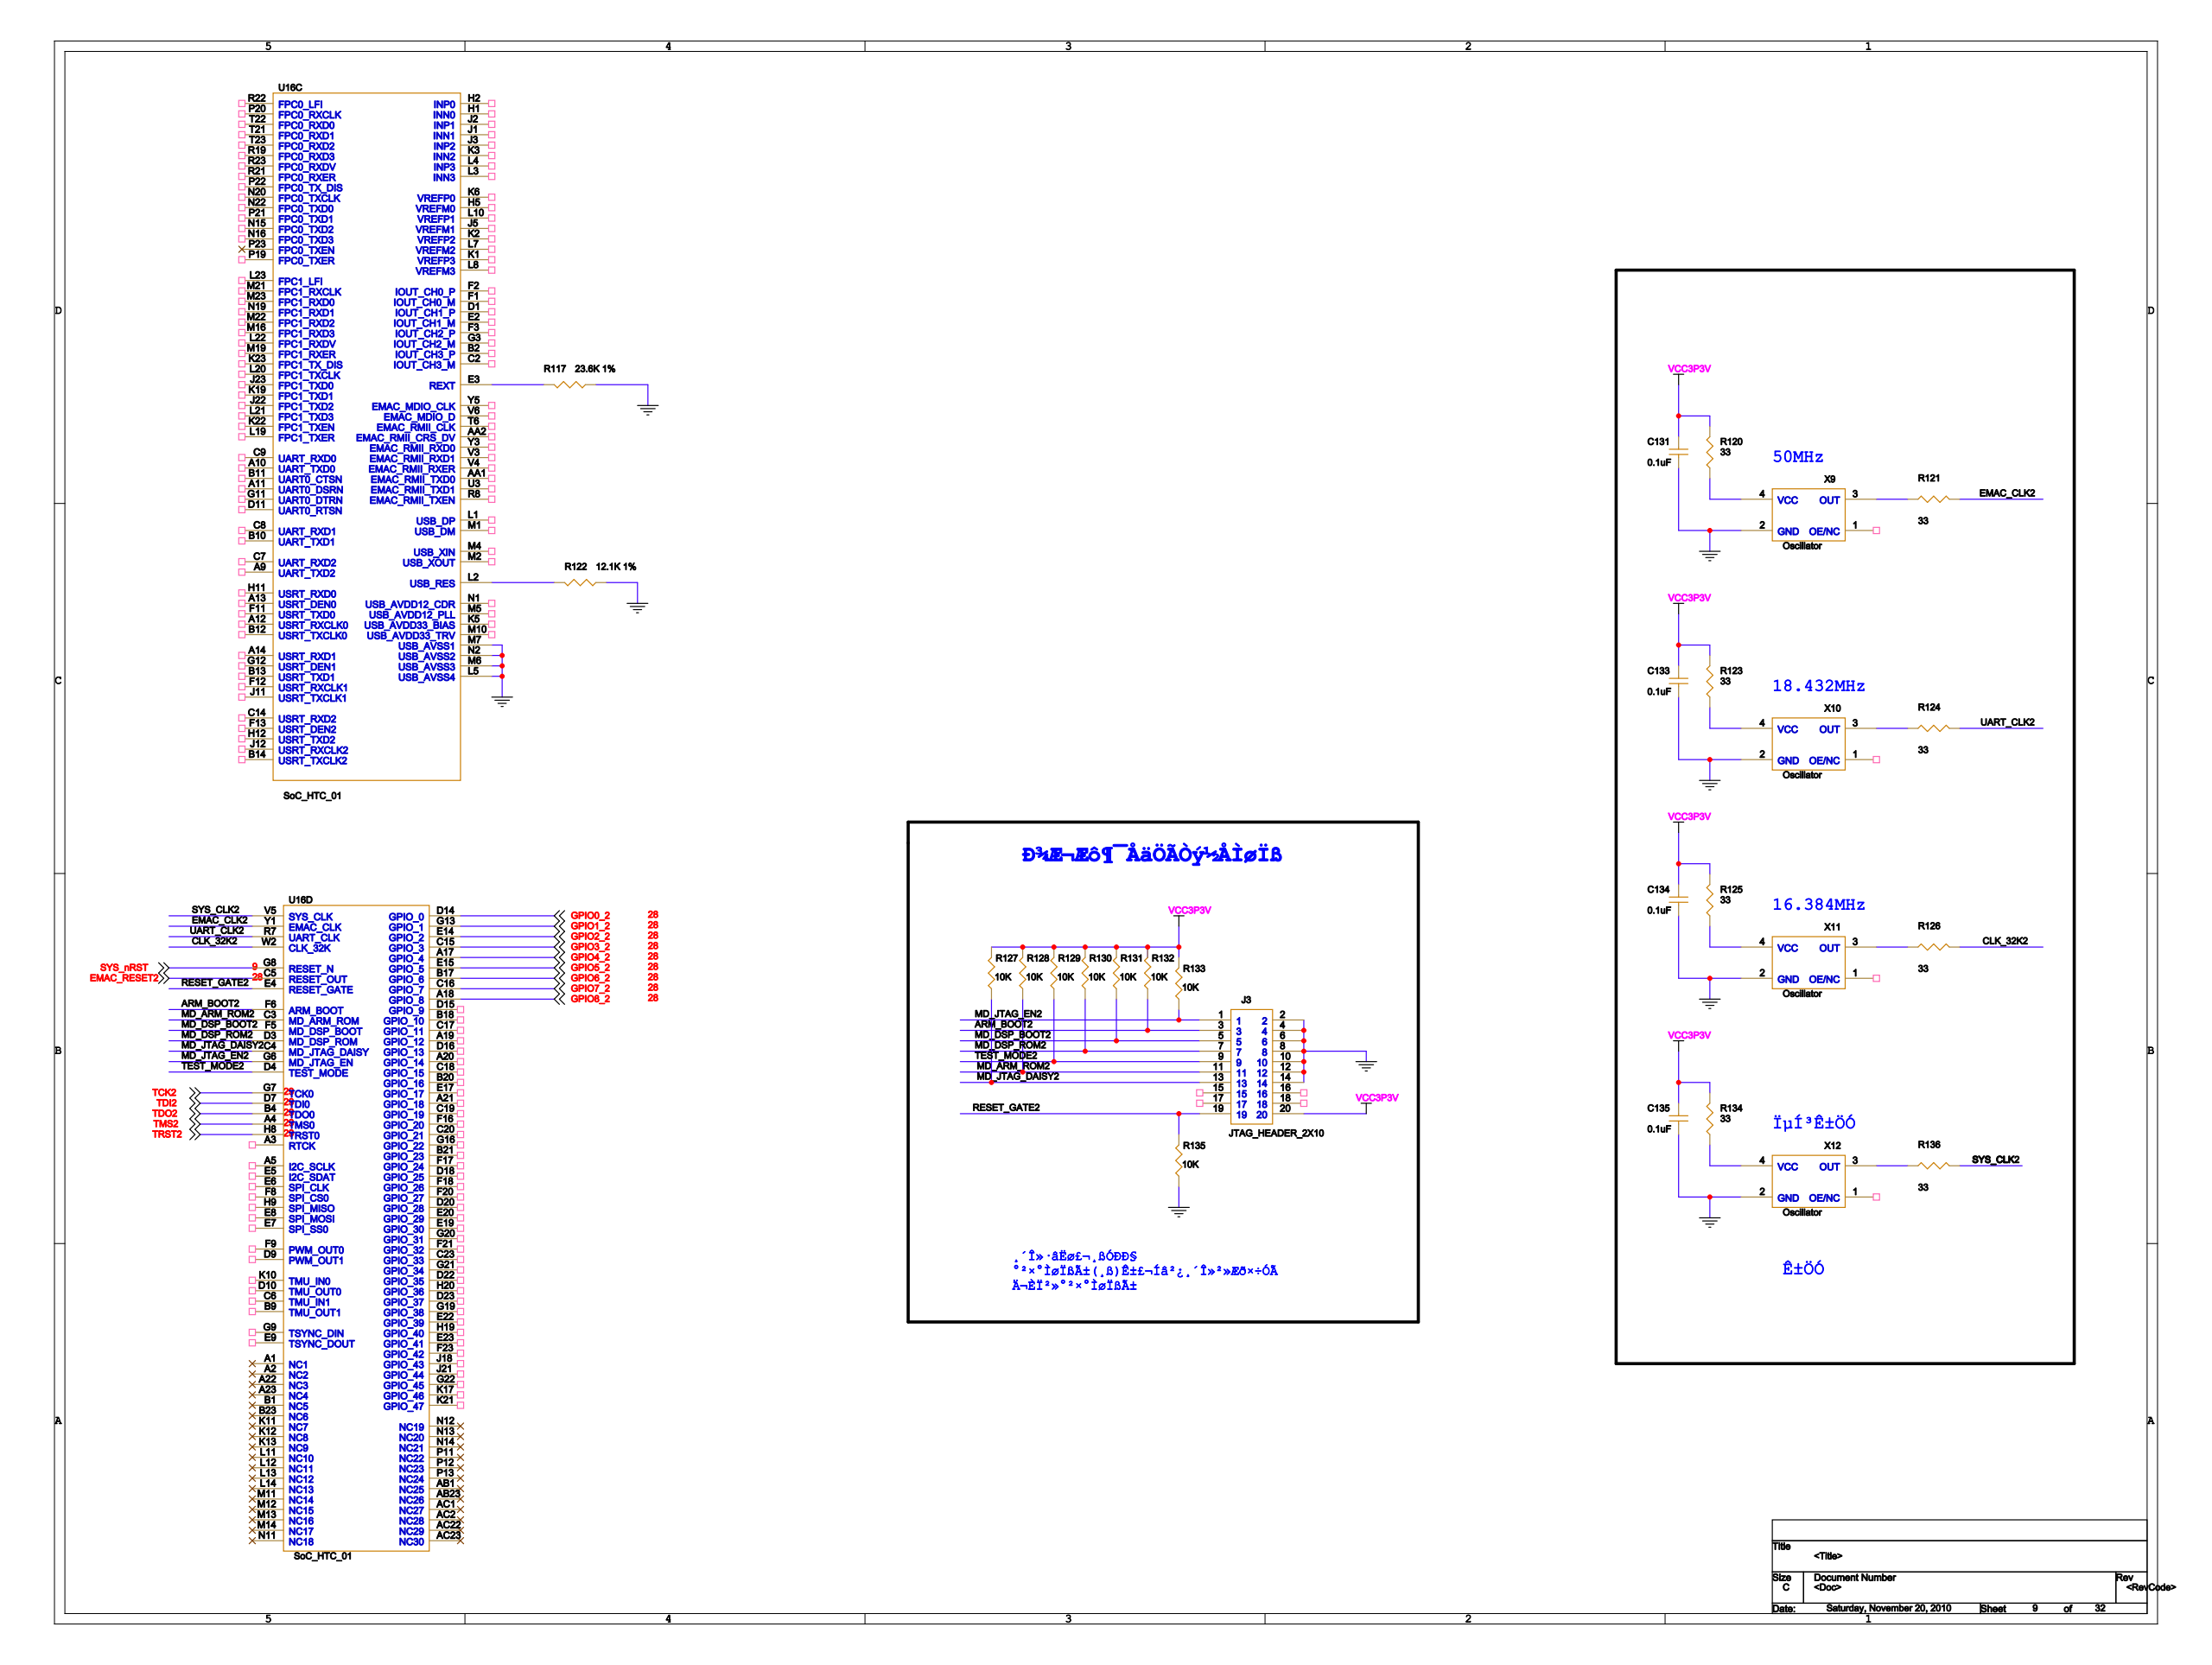Circuit board | Cadence Allegro | 1001 parts | 1318 nets | one sheet of the schematic
Parts on this sheet (reference | value | footprint):
C131 | 0.1uF | 0603
C133 | 0.1uF | 0603
C134 | 0.1uF | 0603
C135 | 0.1uF | 0603
J3 | JTAG_HEADER_2X10 | JTAG_HEADER_2X10
R117 | 23.6K 1% | 0603
R120 | 33 | 0603
R121 | 33 | 0603
R122 | 12.1K 1% | 0603
R123 | 33 | 0603
R124 | 33 | 0603
R125 | 33 | 0603
R126 | 33 | 0603
R127 | 10K | 0603
R128 | 10K | 0603
R129 | 10K | 0603
R130 | 10K | 0603
R131 | 10K | 0603
R132 | 10K | 0603
R133 | 10K | 0603
R134 | 33 | 0603
R135 | 10K | 0603
R136 | 33 | 0603
U16 | SoC_HTC_01 | L529_XIN
X9 | Oscillator | OSC_5_7
X10 | Oscillator | OSC_5_7
X11 | Oscillator | OSC_5_7
X12 | Oscillator | OSC_5_7
Nets of these parts (net: part-pin ...):
GPIO7_2: U16-C16
GPIO0_2: U16-D14
GPIO1_2: U16-G13
TCK2: U16-G7
EMAC_RESET2: U16-C5
GPIO3_2: U16-C15
GPIO2_2: U16-E14
TDI2: U16-D7
TDO2: U16-B4
TMS2: U16-A4
GPIO5_2: U16-E15
TRST2: U16-H8
GPIO4_2: U16-A17
GPIO6_2: U16-B17
GND: C131-2 C133-2 C134-2 C135-2 J3-2 J3-4 J3-6 J3-8 J3-10 J3-12 J3-14 R117-1 R122-1 R135-1 X9-2 X10-2 X11-2 X12-2 U16-L5 U16-M6 U16-M7 U16-N2
GPIO8_2: U16-A18
VCC3P3V: C131-1 C133-1 C134-1 C135-1 J3-20 R120-2 R123-2 R125-2 R127-2 R128-2 R129-2 R130-2 R131-2 R132-2 R133-2 R134-2
N16778458: R117-2 U16-E3
N16778677: R122-2 U16-L2
ARM_BOOT2: J3-3 R132-1 U16-F6
CLK_32K2: R126-2 U16-W2
EMAC_CLK2: R121-2 U16-Y1
MD_ARM_ROM2: J3-11 R128-1 U16-C3
MD_DSP_BOOT2: J3-5 R131-1 U16-F5
MD_DSP_ROM2: J3-7 R130-1 U16-D3
MD_JTAG_DAISY2: J3-13 R127-1 U16-C4
MD_JTAG_EN2: J3-1 R133-1 U16-G6
RESET_GATE2: J3-19 R135-2 U16-E4
SYS_CLK_16778243: R136-2 U16-V5
TEST_MODE2: J3-9 R129-1 U16-D4
UART_CLK2: R124-2 U16-R7
N16778000: R120-1 X9-4
N16778024: R121-1 X9-3
N16778047: R123-1 X10-4
N16778053: R124-1 X10-3
N16778199: R125-1 X11-4
N16778224: R126-1 X11-3
N16778247: R134-1 X12-4
N16778263: R136-1 X12-3